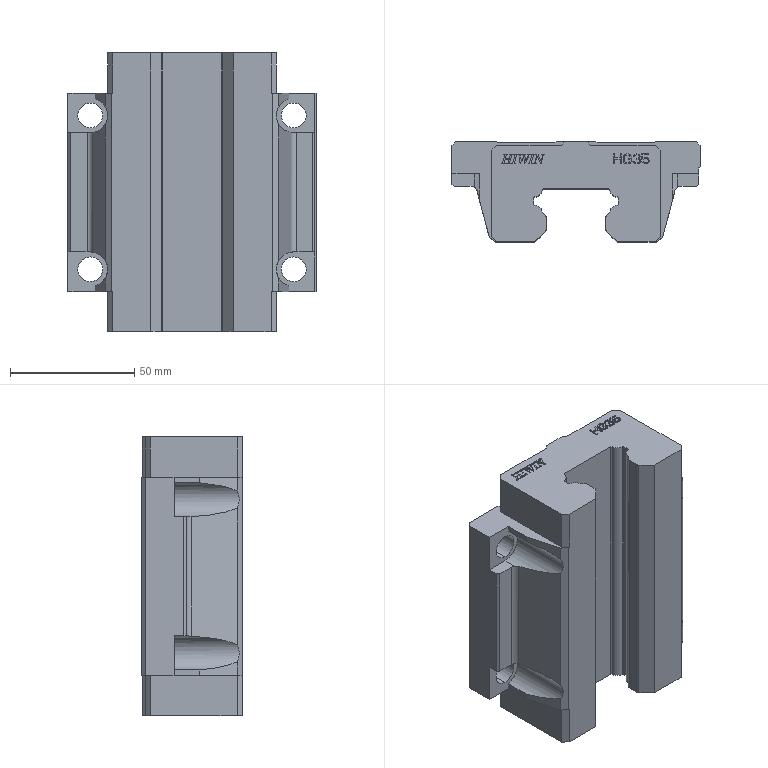Part | SolidWorks | features BaseBody 1 | 1 solid | 397 faces | box 100 x 40.5 x 112.7 mm | volume 283296 mm3 | plane 315 | spline 60 | cylinder 22 | commonest cylinder face diameters 10 x8 2.4 x4 6.5 x4 14 x4 5 x2